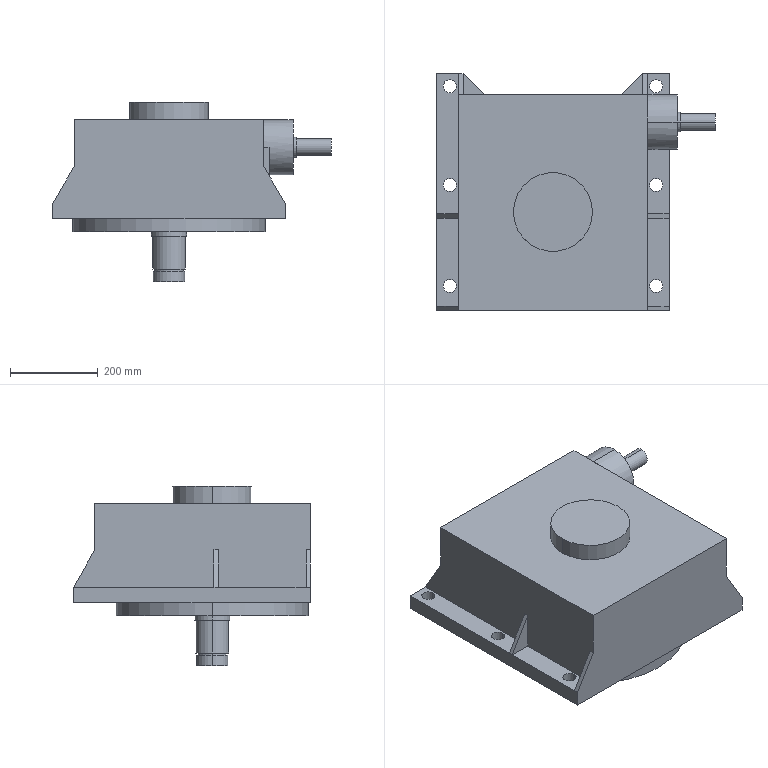Part | SolidWorks | features ICE 15, Extrusion 1, LPattern 1, MirrorPattern 1 | 1 solid | 81 faces | box 635 x 540 x 409 mm | volume 55559758 mm3 | plane 47 | cylinder 34 | commonest cylinder face diameters 30 x12 38 x2 45 x2 65 x2 72 x2 75 x2